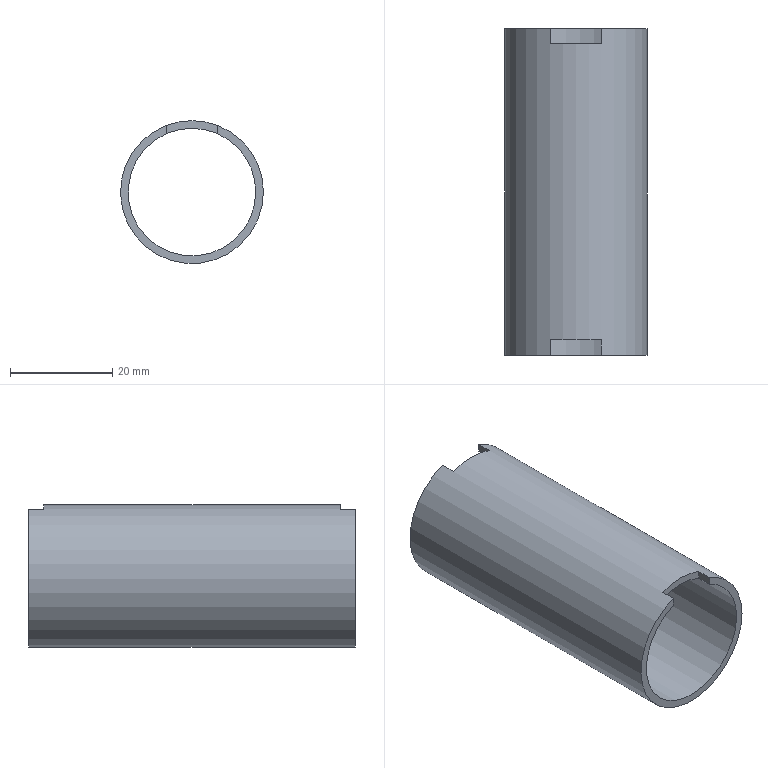Part | STEP file | 1-06.2 | 1 solid | 10 faces | box 28 x 64 x 28 mm | volume 7900 mm3 | plane 8 | cylinder 2 | commonest cylinder face diameters 25 x1 28 x1
STEP:
#1=CARTESIAN_POINT('',(0.,0.,0.));
#2=DIRECTION('',(0.,0.,1.));
#3=DIRECTION('',(1.,0.,0.));
#4=AXIS2_PLACEMENT_3D('',#1,#2,#3);
#5=CARTESIAN_POINT('',(14.,-32.,0.));
#6=VERTEX_POINT('',#5);
#7=CARTESIAN_POINT('',(5.,-32.,13.077));
#8=VERTEX_POINT('',#7);
#9=CARTESIAN_POINT('',(0.,-32.,0.));
#10=DIRECTION('',(0.,-1.,0.));
#11=DIRECTION('',(1.,0.,0.));
#12=AXIS2_PLACEMENT_3D('',#9,#10,#11);
#13=CIRCLE('',#12,14.);
#14=CARTESIAN_POINT('',(-3.751,-32.,0.));
#15=DIRECTION('',(0.,-1.,0.));
#16=DIRECTION('',(1.,0.,0.));
#17=AXIS2_PLACEMENT_3D('',#14,#15,#16);
#18=PLANE('',#17);
#19=CARTESIAN_POINT('',(3.751,0.));
#20=DIRECTION('',(1.,0.));
#21=AXIS2_PLACEMENT_2D('',#19,#20);
#22=CIRCLE('',#21,14.);
#23=(GEOMETRIC_REPRESENTATION_CONTEXT(2)PARAMETRIC_REPRESENTATION_CONTEXT()REPRESENTATION_CONTEXT('',''));
#24=DEFINITIONAL_REPRESENTATION('',(#22),#23);
#25=PCURVE('',#18,#24);
#26=CARTESIAN_POINT('',(0.,-32.,0.));
#27=DIRECTION('',(0.,1.,0.));
#28=DIRECTION('',(1.,0.,0.));
#29=AXIS2_PLACEMENT_3D('',#26,#27,#28);
#30=CYLINDRICAL_SURFACE('',#29,14.);
#31=CARTESIAN_POINT('',(6.283,0.));
#32=DIRECTION('',(-1.,0.));
#33=VECTOR('',#32,1.);
#34=LINE('',#31,#33);
#35=(GEOMETRIC_REPRESENTATION_CONTEXT(2)PARAMETRIC_REPRESENTATION_CONTEXT()REPRESENTATION_CONTEXT('',''));
#36=DEFINITIONAL_REPRESENTATION('',(#34),#35);
#37=PCURVE('',#30,#36);
#38=SURFACE_CURVE('',#13,(#25,#37),.PCURVE_S1.);
#39=EDGE_CURVE('',#6,#8,#38,.T.);
#40=ORIENTED_EDGE('',*,*,#39,.T.);
#41=CARTESIAN_POINT('',(5.,-32.,11.456));
#42=VERTEX_POINT('',#41);
#43=CARTESIAN_POINT('',(5.,-32.,11.456));
#44=DIRECTION('',(0.,0.,1.));
#45=VECTOR('',#44,1.);
#46=LINE('',#43,#45);
#47=CARTESIAN_POINT('',(8.751,11.456));
#48=DIRECTION('',(0.,1.));
#49=VECTOR('',#48,1.);
#50=LINE('',#47,#49);
#51=(GEOMETRIC_REPRESENTATION_CONTEXT(2)PARAMETRIC_REPRESENTATION_CONTEXT()REPRESENTATION_CONTEXT('',''));
#52=DEFINITIONAL_REPRESENTATION('',(#50),#51);
#53=PCURVE('',#18,#52);
#54=CARTESIAN_POINT('',(5.,-30.5,15.));
#55=DIRECTION('',(1.,0.,0.));
#56=DIRECTION('',(0.,1.,0.));
#57=AXIS2_PLACEMENT_3D('',#54,#55,#56);
#58=PLANE('',#57);
#59=CARTESIAN_POINT('',(-1.5,-3.544));
#60=DIRECTION('',(0.,1.));
#61=VECTOR('',#60,1.);
#62=LINE('',#59,#61);
#63=(GEOMETRIC_REPRESENTATION_CONTEXT(2)PARAMETRIC_REPRESENTATION_CONTEXT()REPRESENTATION_CONTEXT('',''));
#64=DEFINITIONAL_REPRESENTATION('',(#62),#63);
#65=PCURVE('',#58,#64);
#66=SURFACE_CURVE('',#46,(#53,#65),.PCURVE_S1.);
#67=EDGE_CURVE('',#42,#8,#66,.T.);
#68=ORIENTED_EDGE('',*,*,#67,.F.);
#69=CARTESIAN_POINT('',(12.5,-32.,0.));
#70=VERTEX_POINT('',#69);
#71=CARTESIAN_POINT('',(0.,-32.,0.));
#72=DIRECTION('',(0.,1.,0.));
#73=DIRECTION('',(0.4,0.,0.9165));
#74=AXIS2_PLACEMENT_3D('',#71,#72,#73);
#75=CIRCLE('',#74,12.5);
#76=CARTESIAN_POINT('',(8.751,11.456));
#77=CARTESIAN_POINT('',(28.594,2.796));
#78=CARTESIAN_POINT('',(11.173,-10.058));
#79=CARTESIAN_POINT('',(-6.249,-22.913));
#80=CARTESIAN_POINT('',(-8.67,-1.398));
#81=CARTESIAN_POINT('',(-11.092,20.117));
#82=CARTESIAN_POINT('',(8.751,11.456));
#83=(BOUNDED_CURVE()B_SPLINE_CURVE(2,(#76,#77,#78,#79,#80,#81,#82),.UNSPECIFIED.,.T.,.F.)B_SPLINE_CURVE_WITH_KNOTS((1,2,2,2,2,1),(-2.094,0.,2.094,4.189,6.283,8.378),.UNSPECIFIED.)CURVE()GEOMETRIC_REPRESENTATION_ITEM()RATIONAL_B_SPLINE_CURVE((1.,0.5,1.,0.5,1.,0.5,1.))REPRESENTATION_ITEM(''));
#84=(GEOMETRIC_REPRESENTATION_CONTEXT(2)PARAMETRIC_REPRESENTATION_CONTEXT()REPRESENTATION_CONTEXT('',''));
#85=DEFINITIONAL_REPRESENTATION('',(#83),#84);
#86=PCURVE('',#18,#85);
#87=CARTESIAN_POINT('',(0.,-32.,0.));
#88=DIRECTION('',(0.,1.,0.));
#89=DIRECTION('',(1.,0.,0.));
#90=AXIS2_PLACEMENT_3D('',#87,#88,#89);
#91=CYLINDRICAL_SURFACE('',#90,12.5);
#92=CARTESIAN_POINT('',(5.124,0.));
#93=DIRECTION('',(1.,0.));
#94=VECTOR('',#93,1.);
#95=LINE('',#92,#94);
#96=(GEOMETRIC_REPRESENTATION_CONTEXT(2)PARAMETRIC_REPRESENTATION_CONTEXT()REPRESENTATION_CONTEXT('',''));
#97=DEFINITIONAL_REPRESENTATION('',(#95),#96);
#98=PCURVE('',#91,#97);
#99=SURFACE_CURVE('',#75,(#86,#98),.PCURVE_S1.);
#100=EDGE_CURVE('',#42,#70,#99,.T.);
#101=ORIENTED_EDGE('',*,*,#100,.T.);
#102=CARTESIAN_POINT('',(-5.,-32.,11.456));
#103=VERTEX_POINT('',#102);
#104=CARTESIAN_POINT('',(0.,-32.,0.));
#105=DIRECTION('',(0.,1.,0.));
#106=DIRECTION('',(1.,0.,0.));
#107=AXIS2_PLACEMENT_3D('',#104,#105,#106);
#108=CIRCLE('',#107,12.5);
#109=CARTESIAN_POINT('',(16.251,0.));
#110=CARTESIAN_POINT('',(16.251,-21.651));
#111=CARTESIAN_POINT('',(-2.499,-10.825));
#112=CARTESIAN_POINT('',(-21.249,0.));
#113=CARTESIAN_POINT('',(-2.499,10.825));
#114=CARTESIAN_POINT('',(16.251,21.651));
#115=CARTESIAN_POINT('',(16.251,0.));
#116=(BOUNDED_CURVE()B_SPLINE_CURVE(2,(#109,#110,#111,#112,#113,#114,#115),.UNSPECIFIED.,.T.,.F.)B_SPLINE_CURVE_WITH_KNOTS((1,2,2,2,2,1),(-2.094,0.,2.094,4.189,6.283,8.378),.UNSPECIFIED.)CURVE()GEOMETRIC_REPRESENTATION_ITEM()RATIONAL_B_SPLINE_CURVE((1.,0.5,1.,0.5,1.,0.5,1.))REPRESENTATION_ITEM(''));
#117=(GEOMETRIC_REPRESENTATION_CONTEXT(2)PARAMETRIC_REPRESENTATION_CONTEXT()REPRESENTATION_CONTEXT('',''));
#118=DEFINITIONAL_REPRESENTATION('',(#116),#117);
#119=PCURVE('',#18,#118);
#120=CARTESIAN_POINT('',(0.,0.));
#121=DIRECTION('',(1.,0.));
#122=VECTOR('',#121,1.);
#123=LINE('',#120,#122);
#124=(GEOMETRIC_REPRESENTATION_CONTEXT(2)PARAMETRIC_REPRESENTATION_CONTEXT()REPRESENTATION_CONTEXT('',''));
#125=DEFINITIONAL_REPRESENTATION('',(#123),#124);
#126=PCURVE('',#91,#125);
#127=SURFACE_CURVE('',#108,(#119,#126),.PCURVE_S1.);
#128=EDGE_CURVE('',#70,#103,#127,.T.);
#129=ORIENTED_EDGE('',*,*,#128,.T.);
#130=CARTESIAN_POINT('',(-5.,-32.,13.077));
#131=VERTEX_POINT('',#130);
#132=CARTESIAN_POINT('',(-5.,-32.,11.456));
#133=DIRECTION('',(0.,0.,1.));
#134=VECTOR('',#133,1.);
#135=LINE('',#132,#134);
#136=CARTESIAN_POINT('',(-1.249,11.456));
#137=DIRECTION('',(0.,1.));
#138=VECTOR('',#137,1.);
#139=LINE('',#136,#138);
#140=(GEOMETRIC_REPRESENTATION_CONTEXT(2)PARAMETRIC_REPRESENTATION_CONTEXT()REPRESENTATION_CONTEXT('',''));
#141=DEFINITIONAL_REPRESENTATION('',(#139),#140);
#142=PCURVE('',#18,#141);
#143=CARTESIAN_POINT('',(-5.,-30.5,15.));
#144=DIRECTION('',(-1.,0.,0.));
#145=DIRECTION('',(0.,-1.,0.));
#146=AXIS2_PLACEMENT_3D('',#143,#144,#145);
#147=PLANE('',#146);
#148=CARTESIAN_POINT('',(1.5,-3.544));
#149=DIRECTION('',(0.,1.));
#150=VECTOR('',#149,1.);
#151=LINE('',#148,#150);
#152=(GEOMETRIC_REPRESENTATION_CONTEXT(2)PARAMETRIC_REPRESENTATION_CONTEXT()REPRESENTATION_CONTEXT('',''));
#153=DEFINITIONAL_REPRESENTATION('',(#151),#152);
#154=PCURVE('',#147,#153);
#155=SURFACE_CURVE('',#135,(#142,#154),.PCURVE_S1.);
#156=EDGE_CURVE('',#103,#131,#155,.T.);
#157=ORIENTED_EDGE('',*,*,#156,.T.);
#158=CARTESIAN_POINT('',(0.,-32.,0.));
#159=DIRECTION('',(0.,-1.,0.));
#160=DIRECTION('',(-0.3571,0.,0.934));
#161=AXIS2_PLACEMENT_3D('',#158,#159,#160);
#162=CIRCLE('',#161,14.);
#163=CARTESIAN_POINT('',(3.751,0.));
#164=DIRECTION('',(-0.3571,0.934));
#165=AXIS2_PLACEMENT_2D('',#163,#164);
#166=CIRCLE('',#165,14.);
#167=(GEOMETRIC_REPRESENTATION_CONTEXT(2)PARAMETRIC_REPRESENTATION_CONTEXT()REPRESENTATION_CONTEXT('',''));
#168=DEFINITIONAL_REPRESENTATION('',(#166),#167);
#169=PCURVE('',#18,#168);
#170=CARTESIAN_POINT('',(4.347,0.));
#171=DIRECTION('',(-1.,0.));
#172=VECTOR('',#171,1.);
#173=LINE('',#170,#172);
#174=(GEOMETRIC_REPRESENTATION_CONTEXT(2)PARAMETRIC_REPRESENTATION_CONTEXT()REPRESENTATION_CONTEXT('',''));
#175=DEFINITIONAL_REPRESENTATION('',(#173),#174);
#176=PCURVE('',#30,#175);
#177=SURFACE_CURVE('',#162,(#169,#176),.PCURVE_S1.);
#178=EDGE_CURVE('',#131,#6,#177,.T.);
#179=ORIENTED_EDGE('',*,*,#178,.T.);
#180=EDGE_LOOP('',(#40,#68,#101,#129,#157,#179));
#181=FACE_BOUND('',#180,.T.);
#182=ADVANCED_FACE('',(#181),#18,.T.);
#183=CARTESIAN_POINT('',(14.,32.,0.));
#184=VERTEX_POINT('',#183);
#185=CARTESIAN_POINT('',(5.,32.,13.077));
#186=VERTEX_POINT('',#185);
#187=CARTESIAN_POINT('',(0.,32.,0.));
#188=DIRECTION('',(0.,-1.,0.));
#189=DIRECTION('',(1.,0.,0.));
#190=AXIS2_PLACEMENT_3D('',#187,#188,#189);
#191=CIRCLE('',#190,14.);
#192=CARTESIAN_POINT('',(-3.751,32.,0.));
#193=DIRECTION('',(0.,-1.,0.));
#194=DIRECTION('',(1.,0.,0.));
#195=AXIS2_PLACEMENT_3D('',#192,#193,#194);
#196=PLANE('',#195);
#197=CARTESIAN_POINT('',(3.751,0.));
#198=DIRECTION('',(1.,0.));
#199=AXIS2_PLACEMENT_2D('',#197,#198);
#200=CIRCLE('',#199,14.);
#201=(GEOMETRIC_REPRESENTATION_CONTEXT(2)PARAMETRIC_REPRESENTATION_CONTEXT()REPRESENTATION_CONTEXT('',''));
#202=DEFINITIONAL_REPRESENTATION('',(#200),#201);
#203=PCURVE('',#196,#202);
#204=CARTESIAN_POINT('',(6.283,64.));
#205=DIRECTION('',(-1.,0.));
#206=VECTOR('',#205,1.);
#207=LINE('',#204,#206);
#208=(GEOMETRIC_REPRESENTATION_CONTEXT(2)PARAMETRIC_REPRESENTATION_CONTEXT()REPRESENTATION_CONTEXT('',''));
#209=DEFINITIONAL_REPRESENTATION('',(#207),#208);
#210=PCURVE('',#30,#209);
#211=SURFACE_CURVE('',#191,(#203,#210),.PCURVE_S1.);
#212=EDGE_CURVE('',#184,#186,#211,.T.);
#213=ORIENTED_EDGE('',*,*,#212,.T.);
#214=CARTESIAN_POINT('',(5.,32.,11.456));
#215=VERTEX_POINT('',#214);
#216=CARTESIAN_POINT('',(5.,32.,11.456));
#217=DIRECTION('',(0.,0.,1.));
#218=VECTOR('',#217,1.);
#219=LINE('',#216,#218);
#220=CARTESIAN_POINT('',(8.751,11.456));
#221=DIRECTION('',(0.,1.));
#222=VECTOR('',#221,1.);
#223=LINE('',#220,#222);
#224=(GEOMETRIC_REPRESENTATION_CONTEXT(2)PARAMETRIC_REPRESENTATION_CONTEXT()REPRESENTATION_CONTEXT('',''));
#225=DEFINITIONAL_REPRESENTATION('',(#223),#224);
#226=PCURVE('',#196,#225);
#227=CARTESIAN_POINT('',(5.,30.5,15.));
#228=DIRECTION('',(1.,0.,0.));
#229=DIRECTION('',(0.,1.,0.));
#230=AXIS2_PLACEMENT_3D('',#227,#228,#229);
#231=PLANE('',#230);
#232=CARTESIAN_POINT('',(1.5,-3.544));
#233=DIRECTION('',(0.,1.));
#234=VECTOR('',#233,1.);
#235=LINE('',#232,#234);
#236=(GEOMETRIC_REPRESENTATION_CONTEXT(2)PARAMETRIC_REPRESENTATION_CONTEXT()REPRESENTATION_CONTEXT('',''));
#237=DEFINITIONAL_REPRESENTATION('',(#235),#236);
#238=PCURVE('',#231,#237);
#239=SURFACE_CURVE('',#219,(#226,#238),.PCURVE_S1.);
#240=EDGE_CURVE('',#215,#186,#239,.T.);
#241=ORIENTED_EDGE('',*,*,#240,.F.);
#242=CARTESIAN_POINT('',(12.5,32.,0.));
#243=VERTEX_POINT('',#242);
#244=CARTESIAN_POINT('',(0.,32.,0.));
#245=DIRECTION('',(0.,1.,0.));
#246=DIRECTION('',(0.4,0.,0.9165));
#247=AXIS2_PLACEMENT_3D('',#244,#245,#246);
#248=CIRCLE('',#247,12.5);
#249=CARTESIAN_POINT('',(8.751,11.456));
#250=CARTESIAN_POINT('',(28.594,2.796));
#251=CARTESIAN_POINT('',(11.173,-10.058));
#252=CARTESIAN_POINT('',(-6.249,-22.913));
#253=CARTESIAN_POINT('',(-8.67,-1.398));
#254=CARTESIAN_POINT('',(-11.092,20.117));
#255=CARTESIAN_POINT('',(8.751,11.456));
#256=(BOUNDED_CURVE()B_SPLINE_CURVE(2,(#249,#250,#251,#252,#253,#254,#255),.UNSPECIFIED.,.T.,.F.)B_SPLINE_CURVE_WITH_KNOTS((1,2,2,2,2,1),(-2.094,0.,2.094,4.189,6.283,8.378),.UNSPECIFIED.)CURVE()GEOMETRIC_REPRESENTATION_ITEM()RATIONAL_B_SPLINE_CURVE((1.,0.5,1.,0.5,1.,0.5,1.))REPRESENTATION_ITEM(''));
#257=(GEOMETRIC_REPRESENTATION_CONTEXT(2)PARAMETRIC_REPRESENTATION_CONTEXT()REPRESENTATION_CONTEXT('',''));
#258=DEFINITIONAL_REPRESENTATION('',(#256),#257);
#259=PCURVE('',#196,#258);
#260=CARTESIAN_POINT('',(5.124,64.));
#261=DIRECTION('',(1.,0.));
#262=VECTOR('',#261,1.);
#263=LINE('',#260,#262);
#264=(GEOMETRIC_REPRESENTATION_CONTEXT(2)PARAMETRIC_REPRESENTATION_CONTEXT()REPRESENTATION_CONTEXT('',''));
#265=DEFINITIONAL_REPRESENTATION('',(#263),#264);
#266=PCURVE('',#91,#265);
#267=SURFACE_CURVE('',#248,(#259,#266),.PCURVE_S1.);
#268=EDGE_CURVE('',#215,#243,#267,.T.);
#269=ORIENTED_EDGE('',*,*,#268,.T.);
#270=CARTESIAN_POINT('',(-5.,32.,11.456));
#271=VERTEX_POINT('',#270);
#272=CARTESIAN_POINT('',(0.,32.,0.));
#273=DIRECTION('',(0.,1.,0.));
#274=DIRECTION('',(1.,0.,0.));
#275=AXIS2_PLACEMENT_3D('',#272,#273,#274);
#276=CIRCLE('',#275,12.5);
#277=CARTESIAN_POINT('',(16.251,0.));
#278=CARTESIAN_POINT('',(16.251,-21.651));
#279=CARTESIAN_POINT('',(-2.499,-10.825));
#280=CARTESIAN_POINT('',(-21.249,0.));
#281=CARTESIAN_POINT('',(-2.499,10.825));
#282=CARTESIAN_POINT('',(16.251,21.651));
#283=CARTESIAN_POINT('',(16.251,0.));
#284=(BOUNDED_CURVE()B_SPLINE_CURVE(2,(#277,#278,#279,#280,#281,#282,#283),.UNSPECIFIED.,.T.,.F.)B_SPLINE_CURVE_WITH_KNOTS((1,2,2,2,2,1),(-2.094,0.,2.094,4.189,6.283,8.378),.UNSPECIFIED.)CURVE()GEOMETRIC_REPRESENTATION_ITEM()RATIONAL_B_SPLINE_CURVE((1.,0.5,1.,0.5,1.,0.5,1.))REPRESENTATION_ITEM(''));
#285=(GEOMETRIC_REPRESENTATION_CONTEXT(2)PARAMETRIC_REPRESENTATION_CONTEXT()REPRESENTATION_CONTEXT('',''));
#286=DEFINITIONAL_REPRESENTATION('',(#284),#285);
#287=PCURVE('',#196,#286);
#288=CARTESIAN_POINT('',(0.,64.));
#289=DIRECTION('',(1.,0.));
#290=VECTOR('',#289,1.);
#291=LINE('',#288,#290);
#292=(GEOMETRIC_REPRESENTATION_CONTEXT(2)PARAMETRIC_REPRESENTATION_CONTEXT()REPRESENTATION_CONTEXT('',''));
#293=DEFINITIONAL_REPRESENTATION('',(#291),#292);
#294=PCURVE('',#91,#293);
#295=SURFACE_CURVE('',#276,(#287,#294),.PCURVE_S1.);
#296=EDGE_CURVE('',#243,#271,#295,.T.);
#297=ORIENTED_EDGE('',*,*,#296,.T.);
#298=CARTESIAN_POINT('',(-5.,32.,13.077));
#299=VERTEX_POINT('',#298);
#300=CARTESIAN_POINT('',(-5.,32.,11.456));
#301=DIRECTION('',(0.,0.,1.));
#302=VECTOR('',#301,1.);
#303=LINE('',#300,#302);
#304=CARTESIAN_POINT('',(-1.249,11.456));
#305=DIRECTION('',(0.,1.));
#306=VECTOR('',#305,1.);
#307=LINE('',#304,#306);
#308=(GEOMETRIC_REPRESENTATION_CONTEXT(2)PARAMETRIC_REPRESENTATION_CONTEXT()REPRESENTATION_CONTEXT('',''));
#309=DEFINITIONAL_REPRESENTATION('',(#307),#308);
#310=PCURVE('',#196,#309);
#311=CARTESIAN_POINT('',(-5.,30.5,15.));
#312=DIRECTION('',(-1.,0.,0.));
#313=DIRECTION('',(0.,-1.,0.));
#314=AXIS2_PLACEMENT_3D('',#311,#312,#313);
#315=PLANE('',#314);
#316=CARTESIAN_POINT('',(-1.5,-3.544));
#317=DIRECTION('',(0.,1.));
#318=VECTOR('',#317,1.);
#319=LINE('',#316,#318);
#320=(GEOMETRIC_REPRESENTATION_CONTEXT(2)PARAMETRIC_REPRESENTATION_CONTEXT()REPRESENTATION_CONTEXT('',''));
#321=DEFINITIONAL_REPRESENTATION('',(#319),#320);
#322=PCURVE('',#315,#321);
#323=SURFACE_CURVE('',#303,(#310,#322),.PCURVE_S1.);
#324=EDGE_CURVE('',#271,#299,#323,.T.);
#325=ORIENTED_EDGE('',*,*,#324,.T.);
#326=CARTESIAN_POINT('',(0.,32.,0.));
#327=DIRECTION('',(0.,-1.,0.));
#328=DIRECTION('',(-0.3571,0.,0.934));
#329=AXIS2_PLACEMENT_3D('',#326,#327,#328);
#330=CIRCLE('',#329,14.);
#331=CARTESIAN_POINT('',(3.751,0.));
#332=DIRECTION('',(-0.3571,0.934));
#333=AXIS2_PLACEMENT_2D('',#331,#332);
#334=CIRCLE('',#333,14.);
#335=(GEOMETRIC_REPRESENTATION_CONTEXT(2)PARAMETRIC_REPRESENTATION_CONTEXT()REPRESENTATION_CONTEXT('',''));
#336=DEFINITIONAL_REPRESENTATION('',(#334),#335);
#337=PCURVE('',#196,#336);
#338=CARTESIAN_POINT('',(4.347,64.));
#339=DIRECTION('',(-1.,0.));
#340=VECTOR('',#339,1.);
#341=LINE('',#338,#340);
#342=(GEOMETRIC_REPRESENTATION_CONTEXT(2)PARAMETRIC_REPRESENTATION_CONTEXT()REPRESENTATION_CONTEXT('',''));
#343=DEFINITIONAL_REPRESENTATION('',(#341),#342);
#344=PCURVE('',#30,#343);
#345=SURFACE_CURVE('',#330,(#337,#344),.PCURVE_S1.);
#346=EDGE_CURVE('',#299,#184,#345,.T.);
#347=ORIENTED_EDGE('',*,*,#346,.T.);
#348=EDGE_LOOP('',(#213,#241,#269,#297,#325,#347));
#349=FACE_BOUND('',#348,.F.);
#350=ADVANCED_FACE('',(#349),#196,.F.);
#351=CARTESIAN_POINT('',(14.,-32.,0.));
#352=DIRECTION('',(0.,1.,0.));
#353=VECTOR('',#352,1.);
#354=LINE('',#351,#353);
#355=CARTESIAN_POINT('',(6.283,0.));
#356=DIRECTION('',(0.,1.));
#357=VECTOR('',#356,1.);
#358=LINE('',#355,#357);
#359=(GEOMETRIC_REPRESENTATION_CONTEXT(2)PARAMETRIC_REPRESENTATION_CONTEXT()REPRESENTATION_CONTEXT('',''));
#360=DEFINITIONAL_REPRESENTATION('',(#358),#359);
#361=PCURVE('',#30,#360);
#362=CARTESIAN_POINT('',(0.,0.));
#363=DIRECTION('',(0.,1.));
#364=VECTOR('',#363,1.);
#365=LINE('',#362,#364);
#366=(GEOMETRIC_REPRESENTATION_CONTEXT(2)PARAMETRIC_REPRESENTATION_CONTEXT()REPRESENTATION_CONTEXT('',''));
#367=DEFINITIONAL_REPRESENTATION('',(#365),#366);
#368=PCURVE('',#30,#367);
#369=SEAM_CURVE('',#354,(#361,#368),.PCURVE_S1.);
#370=EDGE_CURVE('',#6,#184,#369,.T.);
#371=ORIENTED_EDGE('',*,*,#370,.T.);
#372=ORIENTED_EDGE('',*,*,#212,.T.);
#373=CARTESIAN_POINT('',(5.,29.,13.077));
#374=VERTEX_POINT('',#373);
#375=CARTESIAN_POINT('',(5.,29.,13.077));
#376=DIRECTION('',(0.,1.,0.));
#377=VECTOR('',#376,1.);
#378=LINE('',#375,#377);
#379=CARTESIAN_POINT('',(5.078,61.));
#380=DIRECTION('',(0.,1.));
#381=VECTOR('',#380,1.);
#382=LINE('',#379,#381);
#383=(GEOMETRIC_REPRESENTATION_CONTEXT(2)PARAMETRIC_REPRESENTATION_CONTEXT()REPRESENTATION_CONTEXT('',''));
#384=DEFINITIONAL_REPRESENTATION('',(#382),#383);
#385=PCURVE('',#30,#384);
#386=CARTESIAN_POINT('',(-1.5,-1.923));
#387=DIRECTION('',(1.,0.));
#388=VECTOR('',#387,1.);
#389=LINE('',#386,#388);
#390=(GEOMETRIC_REPRESENTATION_CONTEXT(2)PARAMETRIC_REPRESENTATION_CONTEXT()REPRESENTATION_CONTEXT('',''));
#391=DEFINITIONAL_REPRESENTATION('',(#389),#390);
#392=PCURVE('',#231,#391);
#393=SURFACE_CURVE('',#378,(#385,#392),.PCURVE_S1.);
#394=EDGE_CURVE('',#374,#186,#393,.T.);
#395=ORIENTED_EDGE('',*,*,#394,.F.);
#396=CARTESIAN_POINT('',(-5.,29.,13.077));
#397=VERTEX_POINT('',#396);
#398=CARTESIAN_POINT('',(0.,29.,0.));
#399=DIRECTION('',(0.,1.,0.));
#400=DIRECTION('',(-0.3571,0.,0.934));
#401=AXIS2_PLACEMENT_3D('',#398,#399,#400);
#402=CIRCLE('',#401,14.);
#403=CARTESIAN_POINT('',(4.347,61.));
#404=DIRECTION('',(1.,0.));
#405=VECTOR('',#404,1.);
#406=LINE('',#403,#405);
#407=(GEOMETRIC_REPRESENTATION_CONTEXT(2)PARAMETRIC_REPRESENTATION_CONTEXT()REPRESENTATION_CONTEXT('',''));
#408=DEFINITIONAL_REPRESENTATION('',(#406),#407);
#409=PCURVE('',#30,#408);
#410=CARTESIAN_POINT('',(0.,29.,15.));
#411=DIRECTION('',(0.,-1.,0.));
#412=DIRECTION('',(1.,0.,0.));
#413=AXIS2_PLACEMENT_3D('',#410,#411,#412);
#414=PLANE('',#413);
#415=CARTESIAN_POINT('',(-5.,-1.923));
#416=CARTESIAN_POINT('',(17.65,6.737));
#417=CARTESIAN_POINT('',(13.825,-17.208));
#418=CARTESIAN_POINT('',(10.,-41.153));
#419=CARTESIAN_POINT('',(-8.825,-25.868));
#420=CARTESIAN_POINT('',(-27.65,-10.584));
#421=CARTESIAN_POINT('',(-5.,-1.923));
#422=(BOUNDED_CURVE()B_SPLINE_CURVE(2,(#415,#416,#417,#418,#419,#420,#421),.UNSPECIFIED.,.T.,.F.)B_SPLINE_CURVE_WITH_KNOTS((1,2,2,2,2,1),(-2.094,0.,2.094,4.189,6.283,8.378),.UNSPECIFIED.)CURVE()GEOMETRIC_REPRESENTATION_ITEM()RATIONAL_B_SPLINE_CURVE((1.,0.5,1.,0.5,1.,0.5,1.))REPRESENTATION_ITEM(''));
#423=(GEOMETRIC_REPRESENTATION_CONTEXT(2)PARAMETRIC_REPRESENTATION_CONTEXT()REPRESENTATION_CONTEXT('',''));
#424=DEFINITIONAL_REPRESENTATION('',(#422),#423);
#425=PCURVE('',#414,#424);
#426=SURFACE_CURVE('',#402,(#409,#425),.PCURVE_S1.);
#427=EDGE_CURVE('',#397,#374,#426,.T.);
#428=ORIENTED_EDGE('',*,*,#427,.F.);
#429=CARTESIAN_POINT('',(-5.,32.,13.077));
#430=DIRECTION('',(0.,-1.,0.));
#431=VECTOR('',#430,1.);
#432=LINE('',#429,#431);
#433=CARTESIAN_POINT('',(4.347,64.));
#434=DIRECTION('',(0.,-1.));
#435=VECTOR('',#434,1.);
#436=LINE('',#433,#435);
#437=(GEOMETRIC_REPRESENTATION_CONTEXT(2)PARAMETRIC_REPRESENTATION_CONTEXT()REPRESENTATION_CONTEXT('',''));
#438=DEFINITIONAL_REPRESENTATION('',(#436),#437);
#439=PCURVE('',#30,#438);
#440=CARTESIAN_POINT('',(-1.5,-1.923));
#441=DIRECTION('',(1.,0.));
#442=VECTOR('',#441,1.);
#443=LINE('',#440,#442);
#444=(GEOMETRIC_REPRESENTATION_CONTEXT(2)PARAMETRIC_REPRESENTATION_CONTEXT()REPRESENTATION_CONTEXT('',''));
#445=DEFINITIONAL_REPRESENTATION('',(#443),#444);
#446=PCURVE('',#315,#445);
#447=SURFACE_CURVE('',#432,(#439,#446),.PCURVE_S1.);
#448=EDGE_CURVE('',#299,#397,#447,.T.);
#449=ORIENTED_EDGE('',*,*,#448,.F.);
#450=ORIENTED_EDGE('',*,*,#346,.T.);
#451=ORIENTED_EDGE('',*,*,#370,.F.);
#452=ORIENTED_EDGE('',*,*,#178,.F.);
#453=CARTESIAN_POINT('',(-5.,-29.,13.077));
#454=VERTEX_POINT('',#453);
#455=CARTESIAN_POINT('',(-5.,-29.,13.077));
#456=DIRECTION('',(0.,-1.,0.));
#457=VECTOR('',#456,1.);
#458=LINE('',#455,#457);
#459=CARTESIAN_POINT('',(4.347,3.));
#460=DIRECTION('',(0.,-1.));
#461=VECTOR('',#460,1.);
#462=LINE('',#459,#461);
#463=(GEOMETRIC_REPRESENTATION_CONTEXT(2)PARAMETRIC_REPRESENTATION_CONTEXT()REPRESENTATION_CONTEXT('',''));
#464=DEFINITIONAL_REPRESENTATION('',(#462),#463);
#465=PCURVE('',#30,#464);
#466=CARTESIAN_POINT('',(-1.5,-1.923));
#467=DIRECTION('',(1.,0.));
#468=VECTOR('',#467,1.);
#469=LINE('',#466,#468);
#470=(GEOMETRIC_REPRESENTATION_CONTEXT(2)PARAMETRIC_REPRESENTATION_CONTEXT()REPRESENTATION_CONTEXT('',''));
#471=DEFINITIONAL_REPRESENTATION('',(#469),#470);
#472=PCURVE('',#147,#471);
#473=SURFACE_CURVE('',#458,(#465,#472),.PCURVE_S1.);
#474=EDGE_CURVE('',#454,#131,#473,.T.);
#475=ORIENTED_EDGE('',*,*,#474,.F.);
#476=CARTESIAN_POINT('',(5.,-29.,13.077));
#477=VERTEX_POINT('',#476);
#478=CARTESIAN_POINT('',(0.,-29.,0.));
#479=DIRECTION('',(0.,-1.,0.));
#480=DIRECTION('',(0.3571,0.,0.934));
#481=AXIS2_PLACEMENT_3D('',#478,#479,#480);
#482=CIRCLE('',#481,14.);
#483=CARTESIAN_POINT('',(5.078,3.));
#484=DIRECTION('',(-1.,0.));
#485=VECTOR('',#484,1.);
#486=LINE('',#483,#485);
#487=(GEOMETRIC_REPRESENTATION_CONTEXT(2)PARAMETRIC_REPRESENTATION_CONTEXT()REPRESENTATION_CONTEXT('',''));
#488=DEFINITIONAL_REPRESENTATION('',(#486),#487);
#489=PCURVE('',#30,#488);
#490=CARTESIAN_POINT('',(0.,-29.,15.));
#491=DIRECTION('',(0.,1.,0.));
#492=DIRECTION('',(-1.,0.,0.));
#493=AXIS2_PLACEMENT_3D('',#490,#491,#492);
#494=PLANE('',#493);
#495=CARTESIAN_POINT('',(-5.,-1.923));
#496=CARTESIAN_POINT('',(17.65,6.737));
#497=CARTESIAN_POINT('',(13.825,-17.208));
#498=CARTESIAN_POINT('',(10.,-41.153));
#499=CARTESIAN_POINT('',(-8.825,-25.868));
#500=CARTESIAN_POINT('',(-27.65,-10.584));
#501=CARTESIAN_POINT('',(-5.,-1.923));
#502=(BOUNDED_CURVE()B_SPLINE_CURVE(2,(#495,#496,#497,#498,#499,#500,#501),.UNSPECIFIED.,.T.,.F.)B_SPLINE_CURVE_WITH_KNOTS((1,2,2,2,2,1),(-2.094,0.,2.094,4.189,6.283,8.378),.UNSPECIFIED.)CURVE()GEOMETRIC_REPRESENTATION_ITEM()RATIONAL_B_SPLINE_CURVE((1.,0.5,1.,0.5,1.,0.5,1.))REPRESENTATION_ITEM(''));
#503=(GEOMETRIC_REPRESENTATION_CONTEXT(2)PARAMETRIC_REPRESENTATION_CONTEXT()REPRESENTATION_CONTEXT('',''));
#504=DEFINITIONAL_REPRESENTATION('',(#502),#503);
#505=PCURVE('',#494,#504);
#506=SURFACE_CURVE('',#482,(#489,#505),.PCURVE_S1.);
#507=EDGE_CURVE('',#477,#454,#506,.T.);
#508=ORIENTED_EDGE('',*,*,#507,.F.);
#509=CARTESIAN_POINT('',(5.,-32.,13.077));
#510=DIRECTION('',(0.,1.,0.));
#511=VECTOR('',#510,1.);
#512=LINE('',#509,#511);
#513=CARTESIAN_POINT('',(5.078,0.));
#514=DIRECTION('',(0.,1.));
#515=VECTOR('',#514,1.);
#516=LINE('',#513,#515);
#517=(GEOMETRIC_REPRESENTATION_CONTEXT(2)PARAMETRIC_REPRESENTATION_CONTEXT()REPRESENTATION_CONTEXT('',''));
#518=DEFINITIONAL_REPRESENTATION('',(#516),#517);
#519=PCURVE('',#30,#518);
#520=CARTESIAN_POINT('',(-1.5,-1.923));
#521=DIRECTION('',(1.,0.));
#522=VECTOR('',#521,1.);
#523=LINE('',#520,#522);
#524=(GEOMETRIC_REPRESENTATION_CONTEXT(2)PARAMETRIC_REPRESENTATION_CONTEXT()REPRESENTATION_CONTEXT('',''));
#525=DEFINITIONAL_REPRESENTATION('',(#523),#524);
#526=PCURVE('',#58,#525);
#527=SURFACE_CURVE('',#512,(#519,#526),.PCURVE_S1.);
#528=EDGE_CURVE('',#8,#477,#527,.T.);
#529=ORIENTED_EDGE('',*,*,#528,.F.);
#530=ORIENTED_EDGE('',*,*,#39,.F.);
#531=EDGE_LOOP('',(#371,#372,#395,#428,#449,#450,#451,#452,#475,#508,#529,#530));
#532=FACE_BOUND('',#531,.T.);
#533=ADVANCED_FACE('',(#532),#30,.T.);
#534=ORIENTED_EDGE('',*,*,#128,.T.);
#535=CARTESIAN_POINT('',(-5.,-29.,11.456));
#536=VERTEX_POINT('',#535);
#537=CARTESIAN_POINT('',(-5.,-32.,11.456));
#538=DIRECTION('',(0.,1.,0.));
#539=VECTOR('',#538,1.);
#540=LINE('',#537,#539);
#541=CARTESIAN_POINT('',(4.301,0.));
#542=DIRECTION('',(0.,1.));
#543=VECTOR('',#542,1.);
#544=LINE('',#541,#543);
#545=(GEOMETRIC_REPRESENTATION_CONTEXT(2)PARAMETRIC_REPRESENTATION_CONTEXT()REPRESENTATION_CONTEXT('',''));
#546=DEFINITIONAL_REPRESENTATION('',(#544),#545);
#547=PCURVE('',#91,#546);
#548=CARTESIAN_POINT('',(1.5,-3.544));
#549=DIRECTION('',(-1.,0.));
#550=VECTOR('',#549,1.);
#551=LINE('',#548,#550);
#552=(GEOMETRIC_REPRESENTATION_CONTEXT(2)PARAMETRIC_REPRESENTATION_CONTEXT()REPRESENTATION_CONTEXT('',''));
#553=DEFINITIONAL_REPRESENTATION('',(#551),#552);
#554=PCURVE('',#147,#553);
#555=SURFACE_CURVE('',#540,(#547,#554),.PCURVE_S1.);
#556=EDGE_CURVE('',#103,#536,#555,.T.);
#557=ORIENTED_EDGE('',*,*,#556,.T.);
#558=CARTESIAN_POINT('',(5.,-29.,11.456));
#559=VERTEX_POINT('',#558);
#560=CARTESIAN_POINT('',(0.,-29.,0.));
#561=DIRECTION('',(0.,1.,0.));
#562=DIRECTION('',(-0.4,0.,0.9165));
#563=AXIS2_PLACEMENT_3D('',#560,#561,#562);
#564=CIRCLE('',#563,12.5);
#565=CARTESIAN_POINT('',(4.301,3.));
#566=DIRECTION('',(1.,0.));
#567=VECTOR('',#566,1.);
#568=LINE('',#565,#567);
#569=(GEOMETRIC_REPRESENTATION_CONTEXT(2)PARAMETRIC_REPRESENTATION_CONTEXT()REPRESENTATION_CONTEXT('',''));
#570=DEFINITIONAL_REPRESENTATION('',(#568),#569);
#571=PCURVE('',#91,#570);
#572=CARTESIAN_POINT('',(0.,-15.));
#573=DIRECTION('',(0.4,0.9165));
#574=AXIS2_PLACEMENT_2D('',#572,#573);
#575=CIRCLE('',#574,12.5);
#576=(GEOMETRIC_REPRESENTATION_CONTEXT(2)PARAMETRIC_REPRESENTATION_CONTEXT()REPRESENTATION_CONTEXT('',''));
#577=DEFINITIONAL_REPRESENTATION('',(#575),#576);
#578=PCURVE('',#494,#577);
#579=SURFACE_CURVE('',#564,(#571,#578),.PCURVE_S1.);
#580=EDGE_CURVE('',#536,#559,#579,.T.);
#581=ORIENTED_EDGE('',*,*,#580,.T.);
#582=CARTESIAN_POINT('',(5.,-29.,11.456));
#583=DIRECTION('',(0.,-1.,0.));
#584=VECTOR('',#583,1.);
#585=LINE('',#582,#584);
#586=CARTESIAN_POINT('',(5.124,3.));
#587=DIRECTION('',(0.,-1.));
#588=VECTOR('',#587,1.);
#589=LINE('',#586,#588);
#590=(GEOMETRIC_REPRESENTATION_CONTEXT(2)PARAMETRIC_REPRESENTATION_CONTEXT()REPRESENTATION_CONTEXT('',''));
#591=DEFINITIONAL_REPRESENTATION('',(#589),#590);
#592=PCURVE('',#91,#591);
#593=CARTESIAN_POINT('',(1.5,-3.544));
#594=DIRECTION('',(-1.,0.));
#595=VECTOR('',#594,1.);
#596=LINE('',#593,#595);
#597=(GEOMETRIC_REPRESENTATION_CONTEXT(2)PARAMETRIC_REPRESENTATION_CONTEXT()REPRESENTATION_CONTEXT('',''));
#598=DEFINITIONAL_REPRESENTATION('',(#596),#597);
#599=PCURVE('',#58,#598);
#600=SURFACE_CURVE('',#585,(#592,#599),.PCURVE_S1.);
#601=EDGE_CURVE('',#559,#42,#600,.T.);
#602=ORIENTED_EDGE('',*,*,#601,.T.);
#603=ORIENTED_EDGE('',*,*,#100,.T.);
#604=CARTESIAN_POINT('',(12.5,-32.,0.));
#605=DIRECTION('',(0.,1.,0.));
#606=VECTOR('',#605,1.);
#607=LINE('',#604,#606);
#608=CARTESIAN_POINT('',(6.283,0.));
#609=DIRECTION('',(0.,1.));
#610=VECTOR('',#609,1.);
#611=LINE('',#608,#610);
#612=(GEOMETRIC_REPRESENTATION_CONTEXT(2)PARAMETRIC_REPRESENTATION_CONTEXT()REPRESENTATION_CONTEXT('',''));
#613=DEFINITIONAL_REPRESENTATION('',(#611),#612);
#614=PCURVE('',#91,#613);
#615=CARTESIAN_POINT('',(0.,0.));
#616=DIRECTION('',(0.,1.));
#617=VECTOR('',#616,1.);
#618=LINE('',#615,#617);
#619=(GEOMETRIC_REPRESENTATION_CONTEXT(2)PARAMETRIC_REPRESENTATION_CONTEXT()REPRESENTATION_CONTEXT('',''));
#620=DEFINITIONAL_REPRESENTATION('',(#618),#619);
#621=PCURVE('',#91,#620);
#622=SEAM_CURVE('',#607,(#614,#621),.PCURVE_S1.);
#623=EDGE_CURVE('',#70,#243,#622,.T.);
#624=ORIENTED_EDGE('',*,*,#623,.T.);
#625=ORIENTED_EDGE('',*,*,#268,.F.);
#626=CARTESIAN_POINT('',(5.,29.,11.456));
#627=VERTEX_POINT('',#626);
#628=CARTESIAN_POINT('',(5.,32.,11.456));
#629=DIRECTION('',(0.,-1.,0.));
#630=VECTOR('',#629,1.);
#631=LINE('',#628,#630);
#632=CARTESIAN_POINT('',(5.124,64.));
#633=DIRECTION('',(0.,-1.));
#634=VECTOR('',#633,1.);
#635=LINE('',#632,#634);
#636=(GEOMETRIC_REPRESENTATION_CONTEXT(2)PARAMETRIC_REPRESENTATION_CONTEXT()REPRESENTATION_CONTEXT('',''));
#637=DEFINITIONAL_REPRESENTATION('',(#635),#636);
#638=PCURVE('',#91,#637);
#639=CARTESIAN_POINT('',(1.5,-3.544));
#640=DIRECTION('',(-1.,0.));
#641=VECTOR('',#640,1.);
#642=LINE('',#639,#641);
#643=(GEOMETRIC_REPRESENTATION_CONTEXT(2)PARAMETRIC_REPRESENTATION_CONTEXT()REPRESENTATION_CONTEXT('',''));
#644=DEFINITIONAL_REPRESENTATION('',(#642),#643);
#645=PCURVE('',#231,#644);
#646=SURFACE_CURVE('',#631,(#638,#645),.PCURVE_S1.);
#647=EDGE_CURVE('',#215,#627,#646,.T.);
#648=ORIENTED_EDGE('',*,*,#647,.T.);
#649=CARTESIAN_POINT('',(-5.,29.,11.456));
#650=VERTEX_POINT('',#649);
#651=CARTESIAN_POINT('',(0.,29.,0.));
#652=DIRECTION('',(0.,-1.,0.));
#653=DIRECTION('',(0.4,0.,0.9165));
#654=AXIS2_PLACEMENT_3D('',#651,#652,#653);
#655=CIRCLE('',#654,12.5);
#656=CARTESIAN_POINT('',(5.124,61.));
#657=DIRECTION('',(-1.,0.));
#658=VECTOR('',#657,1.);
#659=LINE('',#656,#658);
#660=(GEOMETRIC_REPRESENTATION_CONTEXT(2)PARAMETRIC_REPRESENTATION_CONTEXT()REPRESENTATION_CONTEXT('',''));
#661=DEFINITIONAL_REPRESENTATION('',(#659),#660);
#662=PCURVE('',#91,#661);
#663=CARTESIAN_POINT('',(0.,-15.));
#664=DIRECTION('',(0.4,0.9165));
#665=AXIS2_PLACEMENT_2D('',#663,#664);
#666=CIRCLE('',#665,12.5);
#667=(GEOMETRIC_REPRESENTATION_CONTEXT(2)PARAMETRIC_REPRESENTATION_CONTEXT()REPRESENTATION_CONTEXT('',''));
#668=DEFINITIONAL_REPRESENTATION('',(#666),#667);
#669=PCURVE('',#414,#668);
#670=SURFACE_CURVE('',#655,(#662,#669),.PCURVE_S1.);
#671=EDGE_CURVE('',#627,#650,#670,.T.);
#672=ORIENTED_EDGE('',*,*,#671,.T.);
#673=CARTESIAN_POINT('',(-5.,29.,11.456));
#674=DIRECTION('',(0.,1.,0.));
#675=VECTOR('',#674,1.);
#676=LINE('',#673,#675);
#677=CARTESIAN_POINT('',(4.301,61.));
#678=DIRECTION('',(0.,1.));
#679=VECTOR('',#678,1.);
#680=LINE('',#677,#679);
#681=(GEOMETRIC_REPRESENTATION_CONTEXT(2)PARAMETRIC_REPRESENTATION_CONTEXT()REPRESENTATION_CONTEXT('',''));
#682=DEFINITIONAL_REPRESENTATION('',(#680),#681);
#683=PCURVE('',#91,#682);
#684=CARTESIAN_POINT('',(1.5,-3.544));
#685=DIRECTION('',(-1.,0.));
#686=VECTOR('',#685,1.);
#687=LINE('',#684,#686);
#688=(GEOMETRIC_REPRESENTATION_CONTEXT(2)PARAMETRIC_REPRESENTATION_CONTEXT()REPRESENTATION_CONTEXT('',''));
#689=DEFINITIONAL_REPRESENTATION('',(#687),#688);
#690=PCURVE('',#315,#689);
#691=SURFACE_CURVE('',#676,(#683,#690),.PCURVE_S1.);
#692=EDGE_CURVE('',#650,#271,#691,.T.);
#693=ORIENTED_EDGE('',*,*,#692,.T.);
#694=ORIENTED_EDGE('',*,*,#296,.F.);
#695=ORIENTED_EDGE('',*,*,#623,.F.);
#696=EDGE_LOOP('',(#534,#557,#581,#602,#603,#624,#625,#648,#672,#693,#694,#695));
#697=FACE_BOUND('',#696,.F.);
#698=ADVANCED_FACE('',(#697),#91,.F.);
#699=ORIENTED_EDGE('',*,*,#67,.F.);
#700=ORIENTED_EDGE('',*,*,#601,.F.);
#701=CARTESIAN_POINT('',(5.,-29.,11.456));
#702=DIRECTION('',(0.,0.,1.));
#703=VECTOR('',#702,1.);
#704=LINE('',#701,#703);
#705=CARTESIAN_POINT('',(1.5,-3.544));
#706=DIRECTION('',(0.,1.));
#707=VECTOR('',#706,1.);
#708=LINE('',#705,#707);
#709=(GEOMETRIC_REPRESENTATION_CONTEXT(2)PARAMETRIC_REPRESENTATION_CONTEXT()REPRESENTATION_CONTEXT('',''));
#710=DEFINITIONAL_REPRESENTATION('',(#708),#709);
#711=PCURVE('',#58,#710);
#712=CARTESIAN_POINT('',(-5.,-3.544));
#713=DIRECTION('',(0.,1.));
#714=VECTOR('',#713,1.);
#715=LINE('',#712,#714);
#716=(GEOMETRIC_REPRESENTATION_CONTEXT(2)PARAMETRIC_REPRESENTATION_CONTEXT()REPRESENTATION_CONTEXT('',''));
#717=DEFINITIONAL_REPRESENTATION('',(#715),#716);
#718=PCURVE('',#494,#717);
#719=SURFACE_CURVE('',#704,(#711,#718),.PCURVE_S1.);
#720=EDGE_CURVE('',#559,#477,#719,.T.);
#721=ORIENTED_EDGE('',*,*,#720,.T.);
#722=ORIENTED_EDGE('',*,*,#528,.F.);
#723=EDGE_LOOP('',(#699,#700,#721,#722));
#724=FACE_BOUND('',#723,.F.);
#725=ADVANCED_FACE('',(#724),#58,.F.);
#726=ORIENTED_EDGE('',*,*,#156,.T.);
#727=ORIENTED_EDGE('',*,*,#474,.F.);
#728=CARTESIAN_POINT('',(-5.,-29.,11.456));
#729=DIRECTION('',(0.,0.,1.));
#730=VECTOR('',#729,1.);
#731=LINE('',#728,#730);
#732=CARTESIAN_POINT('',(-1.5,-3.544));
#733=DIRECTION('',(0.,1.));
#734=VECTOR('',#733,1.);
#735=LINE('',#732,#734);
#736=(GEOMETRIC_REPRESENTATION_CONTEXT(2)PARAMETRIC_REPRESENTATION_CONTEXT()REPRESENTATION_CONTEXT('',''));
#737=DEFINITIONAL_REPRESENTATION('',(#735),#736);
#738=PCURVE('',#147,#737);
#739=CARTESIAN_POINT('',(5.,-3.544));
#740=DIRECTION('',(0.,1.));
#741=VECTOR('',#740,1.);
#742=LINE('',#739,#741);
#743=(GEOMETRIC_REPRESENTATION_CONTEXT(2)PARAMETRIC_REPRESENTATION_CONTEXT()REPRESENTATION_CONTEXT('',''));
#744=DEFINITIONAL_REPRESENTATION('',(#742),#743);
#745=PCURVE('',#494,#744);
#746=SURFACE_CURVE('',#731,(#738,#745),.PCURVE_S1.);
#747=EDGE_CURVE('',#536,#454,#746,.T.);
#748=ORIENTED_EDGE('',*,*,#747,.F.);
#749=ORIENTED_EDGE('',*,*,#556,.F.);
#750=EDGE_LOOP('',(#726,#727,#748,#749));
#751=FACE_BOUND('',#750,.F.);
#752=ADVANCED_FACE('',(#751),#147,.F.);
#753=ORIENTED_EDGE('',*,*,#747,.T.);
#754=ORIENTED_EDGE('',*,*,#507,.F.);
#755=ORIENTED_EDGE('',*,*,#720,.F.);
#756=ORIENTED_EDGE('',*,*,#580,.F.);
#757=EDGE_LOOP('',(#753,#754,#755,#756));
#758=FACE_BOUND('',#757,.F.);
#759=ADVANCED_FACE('',(#758),#494,.F.);
#760=CARTESIAN_POINT('',(-5.,29.,11.456));
#761=DIRECTION('',(0.,0.,1.));
#762=VECTOR('',#761,1.);
#763=LINE('',#760,#762);
#764=CARTESIAN_POINT('',(1.5,-3.544));
#765=DIRECTION('',(0.,1.));
#766=VECTOR('',#765,1.);
#767=LINE('',#764,#766);
#768=(GEOMETRIC_REPRESENTATION_CONTEXT(2)PARAMETRIC_REPRESENTATION_CONTEXT()REPRESENTATION_CONTEXT('',''));
#769=DEFINITIONAL_REPRESENTATION('',(#767),#768);
#770=PCURVE('',#315,#769);
#771=CARTESIAN_POINT('',(-5.,-3.544));
#772=DIRECTION('',(0.,1.));
#773=VECTOR('',#772,1.);
#774=LINE('',#771,#773);
#775=(GEOMETRIC_REPRESENTATION_CONTEXT(2)PARAMETRIC_REPRESENTATION_CONTEXT()REPRESENTATION_CONTEXT('',''));
#776=DEFINITIONAL_REPRESENTATION('',(#774),#775);
#777=PCURVE('',#414,#776);
#778=SURFACE_CURVE('',#763,(#770,#777),.PCURVE_S1.);
#779=EDGE_CURVE('',#650,#397,#778,.T.);
#780=ORIENTED_EDGE('',*,*,#779,.T.);
#781=ORIENTED_EDGE('',*,*,#448,.F.);
#782=ORIENTED_EDGE('',*,*,#324,.F.);
#783=ORIENTED_EDGE('',*,*,#692,.F.);
#784=EDGE_LOOP('',(#780,#781,#782,#783));
#785=FACE_BOUND('',#784,.F.);
#786=ADVANCED_FACE('',(#785),#315,.F.);
#787=CARTESIAN_POINT('',(5.,29.,11.456));
#788=DIRECTION('',(0.,0.,1.));
#789=VECTOR('',#788,1.);
#790=LINE('',#787,#789);
#791=CARTESIAN_POINT('',(5.,-3.544));
#792=DIRECTION('',(0.,1.));
#793=VECTOR('',#792,1.);
#794=LINE('',#791,#793);
#795=(GEOMETRIC_REPRESENTATION_CONTEXT(2)PARAMETRIC_REPRESENTATION_CONTEXT()REPRESENTATION_CONTEXT('',''));
#796=DEFINITIONAL_REPRESENTATION('',(#794),#795);
#797=PCURVE('',#414,#796);
#798=CARTESIAN_POINT('',(-1.5,-3.544));
#799=DIRECTION('',(0.,1.));
#800=VECTOR('',#799,1.);
#801=LINE('',#798,#800);
#802=(GEOMETRIC_REPRESENTATION_CONTEXT(2)PARAMETRIC_REPRESENTATION_CONTEXT()REPRESENTATION_CONTEXT('',''));
#803=DEFINITIONAL_REPRESENTATION('',(#801),#802);
#804=PCURVE('',#231,#803);
#805=SURFACE_CURVE('',#790,(#797,#804),.PCURVE_S1.);
#806=EDGE_CURVE('',#627,#374,#805,.T.);
#807=ORIENTED_EDGE('',*,*,#806,.T.);
#808=ORIENTED_EDGE('',*,*,#427,.F.);
#809=ORIENTED_EDGE('',*,*,#779,.F.);
#810=ORIENTED_EDGE('',*,*,#671,.F.);
#811=EDGE_LOOP('',(#807,#808,#809,#810));
#812=FACE_BOUND('',#811,.F.);
#813=ADVANCED_FACE('',(#812),#414,.F.);
#814=ORIENTED_EDGE('',*,*,#240,.T.);
#815=ORIENTED_EDGE('',*,*,#394,.F.);
#816=ORIENTED_EDGE('',*,*,#806,.F.);
#817=ORIENTED_EDGE('',*,*,#647,.F.);
#818=EDGE_LOOP('',(#814,#815,#816,#817));
#819=FACE_BOUND('',#818,.F.);
#820=ADVANCED_FACE('',(#819),#231,.F.);
#821=CLOSED_SHELL('',(#182,#350,#533,#698,#725,#752,#759,#786,#813,#820));
#822=MANIFOLD_SOLID_BREP('',#821);
#823=(LENGTH_UNIT()NAMED_UNIT(*)SI_UNIT(.MILLI.,.METRE.));
#824=UNCERTAINTY_MEASURE_WITH_UNIT(LENGTH_MEASURE(0.0000001),#823,'','');
#825=(NAMED_UNIT(*)PLANE_ANGLE_UNIT()SI_UNIT($,.RADIAN.));
#826=(NAMED_UNIT(*)SI_UNIT($,.STERADIAN.)SOLID_ANGLE_UNIT());
#827=(GEOMETRIC_REPRESENTATION_CONTEXT(3)GLOBAL_UNCERTAINTY_ASSIGNED_CONTEXT((#824))GLOBAL_UNIT_ASSIGNED_CONTEXT((#823,#825,#826))REPRESENTATION_CONTEXT('',''));
#828=ADVANCED_BREP_SHAPE_REPRESENTATION('',(#4,#822),#827);